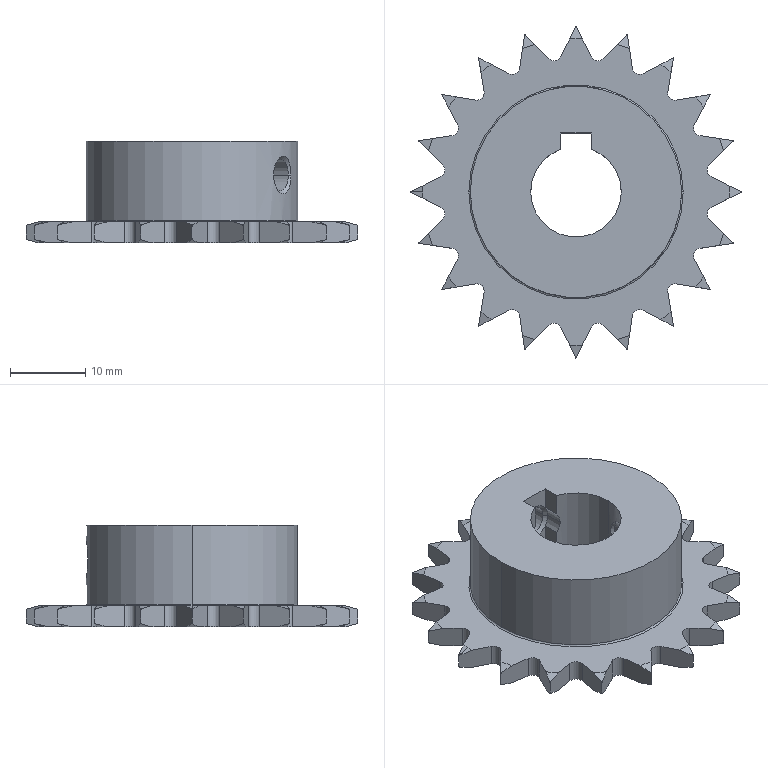Part | SolidWorks | features ICE 3, RevCut 2, Revolution 1 | 1 solid | 187 faces | box 44 x 44 x 13.5 mm | volume 8028 mm3 | cone 53 | plane 49 | torus 44 | cylinder 41 | commonest cylinder face diameters 2 x26 5 x6 4.134 x4 12 x3 28 x2